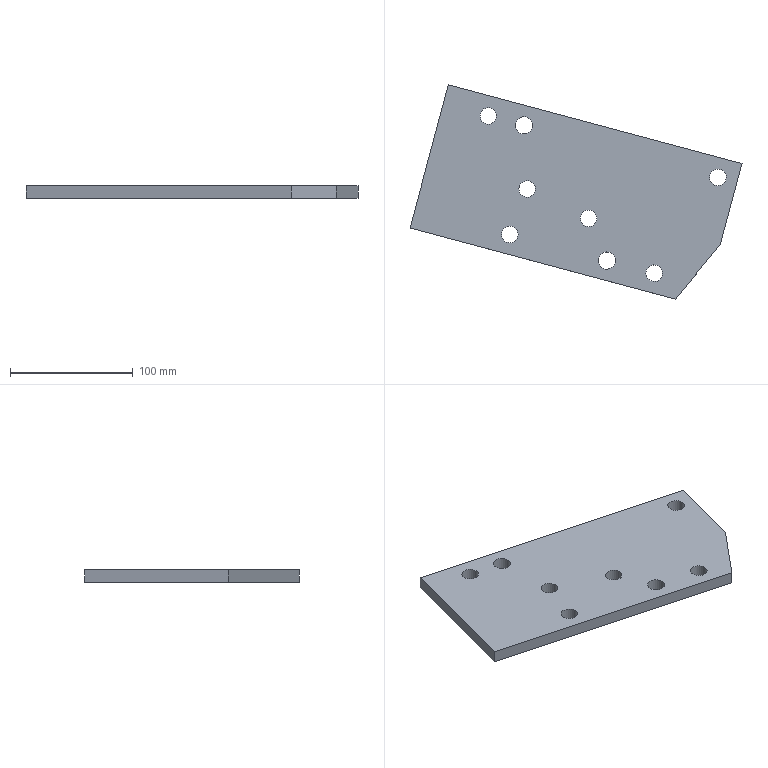Part | NX | features 6 2 | 1 solid | 15 faces | box 270.867 x 174.868 x 10 mm | volume 282148 mm3 | cylinder 8 | plane 7 | commonest cylinder face diameters 13.5 x6 14.001 x2
STEP:
#1=CARTESIAN_POINT('',(347.248,133.494,101.));
#2=VERTEX_POINT('',#1);
#3=CARTESIAN_POINT('',(315.931,16.617,101.));
#4=VERTEX_POINT('',#3);
#5=CARTESIAN_POINT('',(333.53,82.3,101.));
#6=DIRECTION('',(-0.2588,-0.9659,0.));
#7=VECTOR('',#6,1000.);
#8=LINE('',#5,#7);
#9=EDGE_CURVE('',#2,#4,#8,.T.);
#10=ORIENTED_EDGE('',*,*,#9,.T.);
#11=CARTESIAN_POINT('',(532.354,-41.373,101.));
#12=VERTEX_POINT('',#11);
#13=CARTESIAN_POINT('',(446.331,-18.323,101.));
#14=DIRECTION('',(0.9659,-0.2588,0.));
#15=VECTOR('',#14,1000.);
#16=LINE('',#13,#15);
#17=EDGE_CURVE('',#4,#12,#16,.T.);
#18=ORIENTED_EDGE('',*,*,#17,.T.);
#19=CARTESIAN_POINT('',(569.025,2.98,101.));
#20=VERTEX_POINT('',#19);
#21=CARTESIAN_POINT('',(291.39,-332.816,101.));
#22=DIRECTION('',(0.6372,0.7707,0.));
#23=VECTOR('',#22,1000.);
#24=LINE('',#21,#23);
#25=EDGE_CURVE('',#12,#20,#24,.T.);
#26=ORIENTED_EDGE('',*,*,#25,.T.);
#27=CARTESIAN_POINT('',(586.797,69.307,101.));
#28=VERTEX_POINT('',#27);
#29=CARTESIAN_POINT('',(573.08,18.113,101.));
#30=DIRECTION('',(0.2588,0.9659,0.));
#31=VECTOR('',#30,1000.);
#32=LINE('',#29,#31);
#33=EDGE_CURVE('',#20,#28,#32,.T.);
#34=ORIENTED_EDGE('',*,*,#33,.T.);
#35=CARTESIAN_POINT('',(477.648,98.554,101.));
#36=DIRECTION('',(-0.9659,0.2588,0.));
#37=VECTOR('',#36,1000.);
#38=LINE('',#35,#37);
#39=EDGE_CURVE('',#28,#2,#38,.T.);
#40=ORIENTED_EDGE('',*,*,#39,.T.);
#41=EDGE_LOOP('',(#10,#18,#26,#34,#40));
#42=FACE_BOUND('',#41,.T.);
#43=CARTESIAN_POINT('',(418.241,48.522,101.));
#44=VERTEX_POINT('',#43);
#45=CARTESIAN_POINT('',(411.491,48.522,101.));
#46=DIRECTION('',(0.,0.,1.));
#47=DIRECTION('',(1.,0.,0.));
#48=AXIS2_PLACEMENT_3D('',#45,#46,#47);
#49=CIRCLE('',#48,6.75);
#50=EDGE_CURVE('',#44,#44,#49,.T.);
#51=ORIENTED_EDGE('',*,*,#50,.F.);
#52=EDGE_LOOP('',(#51));
#53=FACE_BOUND('',#52,.T.);
#54=CARTESIAN_POINT('',(468.441,24.522,101.));
#55=VERTEX_POINT('',#54);
#56=CARTESIAN_POINT('',(461.691,24.522,101.));
#57=DIRECTION('',(0.,0.,1.));
#58=DIRECTION('',(1.,0.,0.));
#59=AXIS2_PLACEMENT_3D('',#56,#57,#58);
#60=CIRCLE('',#59,6.75);
#61=EDGE_CURVE('',#55,#55,#60,.T.);
#62=ORIENTED_EDGE('',*,*,#61,.F.);
#63=EDGE_LOOP('',(#62));
#64=FACE_BOUND('',#63,.T.);
#65=CARTESIAN_POINT('',(483.314,-11.668,101.));
#66=VERTEX_POINT('',#65);
#67=CARTESIAN_POINT('',(476.552,-9.857,101.));
#68=DIRECTION('',(0.,0.,1.));
#69=DIRECTION('',(0.9659,-0.2588,0.));
#70=AXIS2_PLACEMENT_3D('',#67,#68,#69);
#71=CIRCLE('',#70,7.);
#72=EDGE_CURVE('',#66,#66,#71,.T.);
#73=ORIENTED_EDGE('',*,*,#72,.F.);
#74=EDGE_LOOP('',(#73));
#75=FACE_BOUND('',#74,.T.);
#76=CARTESIAN_POINT('',(403.866,9.62,101.));
#77=VERTEX_POINT('',#76);
#78=CARTESIAN_POINT('',(397.346,11.367,101.));
#79=DIRECTION('',(0.,0.,1.));
#80=DIRECTION('',(0.9659,-0.2588,0.));
#81=AXIS2_PLACEMENT_3D('',#78,#79,#80);
#82=CIRCLE('',#81,6.75);
#83=EDGE_CURVE('',#77,#77,#82,.T.);
#84=ORIENTED_EDGE('',*,*,#83,.F.);
#85=EDGE_LOOP('',(#84));
#86=FACE_BOUND('',#85,.T.);
#87=CARTESIAN_POINT('',(521.709,-21.956,101.));
#88=VERTEX_POINT('',#87);
#89=CARTESIAN_POINT('',(515.189,-20.209,101.));
#90=DIRECTION('',(0.,0.,1.));
#91=DIRECTION('',(0.9659,-0.2588,0.));
#92=AXIS2_PLACEMENT_3D('',#89,#90,#91);
#93=CIRCLE('',#92,6.75);
#94=EDGE_CURVE('',#88,#88,#93,.T.);
#95=ORIENTED_EDGE('',*,*,#94,.F.);
#96=EDGE_LOOP('',(#95));
#97=FACE_BOUND('',#96,.T.);
#98=CARTESIAN_POINT('',(386.332,106.457,101.));
#99=VERTEX_POINT('',#98);
#100=CARTESIAN_POINT('',(379.812,108.204,101.));
#101=DIRECTION('',(0.,0.,1.));
#102=DIRECTION('',(0.9659,-0.2588,0.));
#103=AXIS2_PLACEMENT_3D('',#100,#101,#102);
#104=CIRCLE('',#103,6.75);
#105=EDGE_CURVE('',#99,#99,#104,.T.);
#106=ORIENTED_EDGE('',*,*,#105,.F.);
#107=EDGE_LOOP('',(#106));
#108=FACE_BOUND('',#107,.T.);
#109=CARTESIAN_POINT('',(573.721,56.246,101.));
#110=VERTEX_POINT('',#109);
#111=CARTESIAN_POINT('',(567.201,57.993,101.));
#112=DIRECTION('',(0.,0.,1.));
#113=DIRECTION('',(0.9659,-0.2588,0.));
#114=AXIS2_PLACEMENT_3D('',#111,#112,#113);
#115=CIRCLE('',#114,6.75);
#116=EDGE_CURVE('',#110,#110,#115,.T.);
#117=ORIENTED_EDGE('',*,*,#116,.F.);
#118=EDGE_LOOP('',(#117));
#119=FACE_BOUND('',#118,.T.);
#120=CARTESIAN_POINT('',(415.552,98.628,101.));
#121=VERTEX_POINT('',#120);
#122=CARTESIAN_POINT('',(408.79,100.44,101.));
#123=DIRECTION('',(0.,0.,1.));
#124=DIRECTION('',(0.9659,-0.2588,0.));
#125=AXIS2_PLACEMENT_3D('',#122,#123,#124);
#126=CIRCLE('',#125,7.);
#127=EDGE_CURVE('',#121,#121,#126,.T.);
#128=ORIENTED_EDGE('',*,*,#127,.F.);
#129=EDGE_LOOP('',(#128));
#130=FACE_BOUND('',#129,.T.);
#131=CARTESIAN_POINT('',(1.696,-93.298,101.));
#132=DIRECTION('',(0.,0.,1.));
#133=DIRECTION('',(-0.9848,-0.1736,0.));
#134=AXIS2_PLACEMENT_3D('',#131,#132,#133);
#135=PLANE('',#134);
#136=ADVANCED_FACE('',(#42,#53,#64,#75,#86,#97,#108,#119,#130),#135,.T.);
#137=CARTESIAN_POINT('',(532.354,-41.373,91.));
#138=VERTEX_POINT('',#137);
#139=CARTESIAN_POINT('',(315.931,16.617,91.));
#140=VERTEX_POINT('',#139);
#141=CARTESIAN_POINT('',(446.331,-18.323,91.));
#142=DIRECTION('',(-0.9659,0.2588,0.));
#143=VECTOR('',#142,1000.);
#144=LINE('',#141,#143);
#145=EDGE_CURVE('',#138,#140,#144,.T.);
#146=ORIENTED_EDGE('',*,*,#145,.T.);
#147=CARTESIAN_POINT('',(347.248,133.494,91.));
#148=VERTEX_POINT('',#147);
#149=CARTESIAN_POINT('',(333.53,82.3,91.));
#150=DIRECTION('',(0.2588,0.9659,0.));
#151=VECTOR('',#150,1000.);
#152=LINE('',#149,#151);
#153=EDGE_CURVE('',#140,#148,#152,.T.);
#154=ORIENTED_EDGE('',*,*,#153,.T.);
#155=CARTESIAN_POINT('',(586.797,69.307,91.));
#156=VERTEX_POINT('',#155);
#157=CARTESIAN_POINT('',(477.648,98.554,91.));
#158=DIRECTION('',(0.9659,-0.2588,0.));
#159=VECTOR('',#158,1000.);
#160=LINE('',#157,#159);
#161=EDGE_CURVE('',#148,#156,#160,.T.);
#162=ORIENTED_EDGE('',*,*,#161,.T.);
#163=CARTESIAN_POINT('',(569.025,2.98,91.));
#164=VERTEX_POINT('',#163);
#165=CARTESIAN_POINT('',(573.08,18.113,91.));
#166=DIRECTION('',(-0.2588,-0.9659,0.));
#167=VECTOR('',#166,1000.);
#168=LINE('',#165,#167);
#169=EDGE_CURVE('',#156,#164,#168,.T.);
#170=ORIENTED_EDGE('',*,*,#169,.T.);
#171=CARTESIAN_POINT('',(532.646,-41.021,91.));
#172=DIRECTION('',(0.6372,0.7707,0.));
#173=VECTOR('',#172,1000.);
#174=LINE('',#171,#173);
#175=EDGE_CURVE('',#138,#164,#174,.T.);
#176=ORIENTED_EDGE('',*,*,#175,.F.);
#177=EDGE_LOOP('',(#146,#154,#162,#170,#176));
#178=FACE_BOUND('',#177,.T.);
#179=CARTESIAN_POINT('',(415.552,98.628,91.));
#180=VERTEX_POINT('',#179);
#181=CARTESIAN_POINT('',(408.79,100.44,91.));
#182=DIRECTION('',(0.,0.,-1.));
#183=DIRECTION('',(0.9659,-0.2588,0.));
#184=AXIS2_PLACEMENT_3D('',#181,#182,#183);
#185=CIRCLE('',#184,7.);
#186=EDGE_CURVE('',#180,#180,#185,.T.);
#187=ORIENTED_EDGE('',*,*,#186,.F.);
#188=EDGE_LOOP('',(#187));
#189=FACE_BOUND('',#188,.T.);
#190=CARTESIAN_POINT('',(573.721,56.246,91.));
#191=VERTEX_POINT('',#190);
#192=CARTESIAN_POINT('',(567.201,57.993,91.));
#193=DIRECTION('',(0.,0.,-1.));
#194=DIRECTION('',(0.9659,-0.2588,0.));
#195=AXIS2_PLACEMENT_3D('',#192,#193,#194);
#196=CIRCLE('',#195,6.75);
#197=EDGE_CURVE('',#191,#191,#196,.T.);
#198=ORIENTED_EDGE('',*,*,#197,.F.);
#199=EDGE_LOOP('',(#198));
#200=FACE_BOUND('',#199,.T.);
#201=CARTESIAN_POINT('',(386.332,106.457,91.));
#202=VERTEX_POINT('',#201);
#203=CARTESIAN_POINT('',(379.812,108.204,91.));
#204=DIRECTION('',(0.,0.,-1.));
#205=DIRECTION('',(0.9659,-0.2588,0.));
#206=AXIS2_PLACEMENT_3D('',#203,#204,#205);
#207=CIRCLE('',#206,6.75);
#208=EDGE_CURVE('',#202,#202,#207,.T.);
#209=ORIENTED_EDGE('',*,*,#208,.F.);
#210=EDGE_LOOP('',(#209));
#211=FACE_BOUND('',#210,.T.);
#212=CARTESIAN_POINT('',(521.709,-21.956,91.));
#213=VERTEX_POINT('',#212);
#214=CARTESIAN_POINT('',(515.189,-20.209,91.));
#215=DIRECTION('',(0.,0.,-1.));
#216=DIRECTION('',(0.9659,-0.2588,0.));
#217=AXIS2_PLACEMENT_3D('',#214,#215,#216);
#218=CIRCLE('',#217,6.75);
#219=EDGE_CURVE('',#213,#213,#218,.T.);
#220=ORIENTED_EDGE('',*,*,#219,.F.);
#221=EDGE_LOOP('',(#220));
#222=FACE_BOUND('',#221,.T.);
#223=CARTESIAN_POINT('',(403.866,9.62,91.));
#224=VERTEX_POINT('',#223);
#225=CARTESIAN_POINT('',(397.346,11.367,91.));
#226=DIRECTION('',(0.,0.,-1.));
#227=DIRECTION('',(0.9659,-0.2588,0.));
#228=AXIS2_PLACEMENT_3D('',#225,#226,#227);
#229=CIRCLE('',#228,6.75);
#230=EDGE_CURVE('',#224,#224,#229,.T.);
#231=ORIENTED_EDGE('',*,*,#230,.F.);
#232=EDGE_LOOP('',(#231));
#233=FACE_BOUND('',#232,.T.);
#234=CARTESIAN_POINT('',(483.314,-11.668,91.));
#235=VERTEX_POINT('',#234);
#236=CARTESIAN_POINT('',(476.552,-9.857,91.));
#237=DIRECTION('',(0.,0.,-1.));
#238=DIRECTION('',(0.9659,-0.2588,0.));
#239=AXIS2_PLACEMENT_3D('',#236,#237,#238);
#240=CIRCLE('',#239,7.);
#241=EDGE_CURVE('',#235,#235,#240,.T.);
#242=ORIENTED_EDGE('',*,*,#241,.F.);
#243=EDGE_LOOP('',(#242));
#244=FACE_BOUND('',#243,.T.);
#245=CARTESIAN_POINT('',(454.941,24.522,91.));
#246=VERTEX_POINT('',#245);
#247=CARTESIAN_POINT('',(461.691,24.522,91.));
#248=DIRECTION('',(0.,0.,1.));
#249=DIRECTION('',(-1.,0.,0.));
#250=AXIS2_PLACEMENT_3D('',#247,#248,#249);
#251=CIRCLE('',#250,6.75);
#252=EDGE_CURVE('',#246,#246,#251,.T.);
#253=ORIENTED_EDGE('',*,*,#252,.T.);
#254=EDGE_LOOP('',(#253));
#255=FACE_BOUND('',#254,.T.);
#256=CARTESIAN_POINT('',(404.741,48.522,91.));
#257=VERTEX_POINT('',#256);
#258=CARTESIAN_POINT('',(411.491,48.522,91.));
#259=DIRECTION('',(0.,0.,1.));
#260=DIRECTION('',(-1.,0.,0.));
#261=AXIS2_PLACEMENT_3D('',#258,#259,#260);
#262=CIRCLE('',#261,6.75);
#263=EDGE_CURVE('',#257,#257,#262,.T.);
#264=ORIENTED_EDGE('',*,*,#263,.T.);
#265=EDGE_LOOP('',(#264));
#266=FACE_BOUND('',#265,.T.);
#267=CARTESIAN_POINT('',(463.93,47.36,91.));
#268=DIRECTION('',(0.,0.,-1.));
#269=DIRECTION('',(0.9659,-0.2588,0.));
#270=AXIS2_PLACEMENT_3D('',#267,#268,#269);
#271=PLANE('',#270);
#272=ADVANCED_FACE('',(#178,#189,#200,#211,#222,#233,#244,#255,#266),#271,.T.);
#273=ORIENTED_EDGE('',*,*,#17,.F.);
#274=CARTESIAN_POINT('',(315.931,16.617,91.));
#275=DIRECTION('',(0.,0.,1.));
#276=VECTOR('',#275,1000.);
#277=LINE('',#274,#276);
#278=EDGE_CURVE('',#140,#4,#277,.T.);
#279=ORIENTED_EDGE('',*,*,#278,.F.);
#280=ORIENTED_EDGE('',*,*,#145,.F.);
#281=CARTESIAN_POINT('',(532.354,-41.373,-36.));
#282=DIRECTION('',(0.,0.,-1.));
#283=VECTOR('',#282,1000.);
#284=LINE('',#281,#283);
#285=EDGE_CURVE('',#12,#138,#284,.T.);
#286=ORIENTED_EDGE('',*,*,#285,.F.);
#287=EDGE_LOOP('',(#273,#279,#280,#286));
#288=FACE_BOUND('',#287,.T.);
#289=CARTESIAN_POINT('',(446.331,-18.323,91.));
#290=DIRECTION('',(-0.2588,-0.9659,0.));
#291=DIRECTION('',(0.,0.,-1.));
#292=AXIS2_PLACEMENT_3D('',#289,#290,#291);
#293=PLANE('',#292);
#294=ADVANCED_FACE('',(#288),#293,.T.);
#295=ORIENTED_EDGE('',*,*,#153,.F.);
#296=ORIENTED_EDGE('',*,*,#278,.T.);
#297=ORIENTED_EDGE('',*,*,#9,.F.);
#298=CARTESIAN_POINT('',(347.248,133.494,91.));
#299=DIRECTION('',(0.,0.,1.));
#300=VECTOR('',#299,1000.);
#301=LINE('',#298,#300);
#302=EDGE_CURVE('',#148,#2,#301,.T.);
#303=ORIENTED_EDGE('',*,*,#302,.F.);
#304=EDGE_LOOP('',(#295,#296,#297,#303));
#305=FACE_BOUND('',#304,.T.);
#306=CARTESIAN_POINT('',(333.53,82.3,91.));
#307=DIRECTION('',(-0.9659,0.2588,0.));
#308=DIRECTION('',(0.,0.,-1.));
#309=AXIS2_PLACEMENT_3D('',#306,#307,#308);
#310=PLANE('',#309);
#311=ADVANCED_FACE('',(#305),#310,.T.);
#312=ORIENTED_EDGE('',*,*,#302,.T.);
#313=ORIENTED_EDGE('',*,*,#39,.F.);
#314=CARTESIAN_POINT('',(586.797,69.307,91.));
#315=DIRECTION('',(0.,0.,1.));
#316=VECTOR('',#315,1000.);
#317=LINE('',#314,#316);
#318=EDGE_CURVE('',#156,#28,#317,.T.);
#319=ORIENTED_EDGE('',*,*,#318,.F.);
#320=ORIENTED_EDGE('',*,*,#161,.F.);
#321=EDGE_LOOP('',(#312,#313,#319,#320));
#322=FACE_BOUND('',#321,.T.);
#323=CARTESIAN_POINT('',(477.648,98.554,91.));
#324=DIRECTION('',(0.2588,0.9659,0.));
#325=DIRECTION('',(0.,0.,1.));
#326=AXIS2_PLACEMENT_3D('',#323,#324,#325);
#327=PLANE('',#326);
#328=ADVANCED_FACE('',(#322),#327,.T.);
#329=ORIENTED_EDGE('',*,*,#33,.F.);
#330=CARTESIAN_POINT('',(569.025,2.98,-36.));
#331=DIRECTION('',(0.,0.,1.));
#332=VECTOR('',#331,1000.);
#333=LINE('',#330,#332);
#334=EDGE_CURVE('',#164,#20,#333,.T.);
#335=ORIENTED_EDGE('',*,*,#334,.F.);
#336=ORIENTED_EDGE('',*,*,#169,.F.);
#337=ORIENTED_EDGE('',*,*,#318,.T.);
#338=EDGE_LOOP('',(#329,#335,#336,#337));
#339=FACE_BOUND('',#338,.T.);
#340=CARTESIAN_POINT('',(573.08,18.113,91.));
#341=DIRECTION('',(0.9659,-0.2588,0.));
#342=DIRECTION('',(0.,0.,1.));
#343=AXIS2_PLACEMENT_3D('',#340,#341,#342);
#344=PLANE('',#343);
#345=ADVANCED_FACE('',(#339),#344,.T.);
#346=ORIENTED_EDGE('',*,*,#105,.T.);
#347=EDGE_LOOP('',(#346));
#348=FACE_BOUND('',#347,.T.);
#349=ORIENTED_EDGE('',*,*,#208,.T.);
#350=EDGE_LOOP('',(#349));
#351=FACE_BOUND('',#350,.T.);
#352=CARTESIAN_POINT('',(379.812,108.204,91.));
#353=DIRECTION('',(0.,0.,1.));
#354=DIRECTION('',(-0.9659,0.2588,0.));
#355=AXIS2_PLACEMENT_3D('',#352,#353,#354);
#356=CYLINDRICAL_SURFACE('',#355,6.75);
#357=ADVANCED_FACE('',(#348,#351),#356,.F.);
#358=ORIENTED_EDGE('',*,*,#94,.T.);
#359=EDGE_LOOP('',(#358));
#360=FACE_BOUND('',#359,.T.);
#361=ORIENTED_EDGE('',*,*,#219,.T.);
#362=EDGE_LOOP('',(#361));
#363=FACE_BOUND('',#362,.T.);
#364=CARTESIAN_POINT('',(515.189,-20.209,91.));
#365=DIRECTION('',(0.,0.,1.));
#366=DIRECTION('',(-0.9659,0.2588,0.));
#367=AXIS2_PLACEMENT_3D('',#364,#365,#366);
#368=CYLINDRICAL_SURFACE('',#367,6.75);
#369=ADVANCED_FACE('',(#360,#363),#368,.F.);
#370=ORIENTED_EDGE('',*,*,#116,.T.);
#371=EDGE_LOOP('',(#370));
#372=FACE_BOUND('',#371,.T.);
#373=ORIENTED_EDGE('',*,*,#197,.T.);
#374=EDGE_LOOP('',(#373));
#375=FACE_BOUND('',#374,.T.);
#376=CARTESIAN_POINT('',(567.201,57.993,91.));
#377=DIRECTION('',(0.,0.,1.));
#378=DIRECTION('',(-0.9659,0.2588,0.));
#379=AXIS2_PLACEMENT_3D('',#376,#377,#378);
#380=CYLINDRICAL_SURFACE('',#379,6.75);
#381=ADVANCED_FACE('',(#372,#375),#380,.F.);
#382=ORIENTED_EDGE('',*,*,#83,.T.);
#383=EDGE_LOOP('',(#382));
#384=FACE_BOUND('',#383,.T.);
#385=ORIENTED_EDGE('',*,*,#230,.T.);
#386=EDGE_LOOP('',(#385));
#387=FACE_BOUND('',#386,.T.);
#388=CARTESIAN_POINT('',(397.346,11.367,91.));
#389=DIRECTION('',(0.,0.,1.));
#390=DIRECTION('',(-0.9659,0.2588,0.));
#391=AXIS2_PLACEMENT_3D('',#388,#389,#390);
#392=CYLINDRICAL_SURFACE('',#391,6.75);
#393=ADVANCED_FACE('',(#384,#387),#392,.F.);
#394=ORIENTED_EDGE('',*,*,#127,.T.);
#395=EDGE_LOOP('',(#394));
#396=FACE_BOUND('',#395,.T.);
#397=ORIENTED_EDGE('',*,*,#186,.T.);
#398=EDGE_LOOP('',(#397));
#399=FACE_BOUND('',#398,.T.);
#400=CARTESIAN_POINT('',(408.79,100.44,91.));
#401=DIRECTION('',(0.,0.,1.));
#402=DIRECTION('',(-0.9659,0.2588,0.));
#403=AXIS2_PLACEMENT_3D('',#400,#401,#402);
#404=CYLINDRICAL_SURFACE('',#403,7.);
#405=ADVANCED_FACE('',(#396,#399),#404,.F.);
#406=ORIENTED_EDGE('',*,*,#72,.T.);
#407=EDGE_LOOP('',(#406));
#408=FACE_BOUND('',#407,.T.);
#409=ORIENTED_EDGE('',*,*,#241,.T.);
#410=EDGE_LOOP('',(#409));
#411=FACE_BOUND('',#410,.T.);
#412=CARTESIAN_POINT('',(476.552,-9.857,91.));
#413=DIRECTION('',(0.,0.,1.));
#414=DIRECTION('',(-0.9659,0.2588,0.));
#415=AXIS2_PLACEMENT_3D('',#412,#413,#414);
#416=CYLINDRICAL_SURFACE('',#415,7.);
#417=ADVANCED_FACE('',(#408,#411),#416,.F.);
#418=ORIENTED_EDGE('',*,*,#25,.F.);
#419=ORIENTED_EDGE('',*,*,#285,.T.);
#420=ORIENTED_EDGE('',*,*,#175,.T.);
#421=ORIENTED_EDGE('',*,*,#334,.T.);
#422=EDGE_LOOP('',(#418,#419,#420,#421));
#423=FACE_BOUND('',#422,.T.);
#424=CARTESIAN_POINT('',(532.646,-41.021,-36.));
#425=DIRECTION('',(0.7707,-0.6372,0.));
#426=DIRECTION('',(-0.6372,-0.7707,0.));
#427=AXIS2_PLACEMENT_3D('',#424,#425,#426);
#428=PLANE('',#427);
#429=ADVANCED_FACE('',(#423),#428,.T.);
#430=ORIENTED_EDGE('',*,*,#61,.T.);
#431=EDGE_LOOP('',(#430));
#432=FACE_BOUND('',#431,.T.);
#433=ORIENTED_EDGE('',*,*,#252,.F.);
#434=EDGE_LOOP('',(#433));
#435=FACE_BOUND('',#434,.T.);
#436=CARTESIAN_POINT('',(461.691,24.522,-61.));
#437=DIRECTION('',(0.,0.,1.));
#438=DIRECTION('',(-1.,0.,0.));
#439=AXIS2_PLACEMENT_3D('',#436,#437,#438);
#440=CYLINDRICAL_SURFACE('',#439,6.75);
#441=ADVANCED_FACE('',(#432,#435),#440,.F.);
#442=ORIENTED_EDGE('',*,*,#50,.T.);
#443=EDGE_LOOP('',(#442));
#444=FACE_BOUND('',#443,.T.);
#445=ORIENTED_EDGE('',*,*,#263,.F.);
#446=EDGE_LOOP('',(#445));
#447=FACE_BOUND('',#446,.T.);
#448=CARTESIAN_POINT('',(411.491,48.522,-61.));
#449=DIRECTION('',(0.,0.,1.));
#450=DIRECTION('',(-1.,0.,0.));
#451=AXIS2_PLACEMENT_3D('',#448,#449,#450);
#452=CYLINDRICAL_SURFACE('',#451,6.75);
#453=ADVANCED_FACE('',(#444,#447),#452,.F.);
#454=CLOSED_SHELL('',(#136,#272,#294,#311,#328,#345,#357,#369,#381,#393,#405,#417,#429,#441,#453));
#455=MANIFOLD_SOLID_BREP('',#454);
#456=(LENGTH_UNIT()NAMED_UNIT(*)SI_UNIT(.MILLI.,.METRE.));
#457=UNCERTAINTY_MEASURE_WITH_UNIT(LENGTH_MEASURE(0.00001),#456,'','');
#458=(NAMED_UNIT(*)PLANE_ANGLE_UNIT()SI_UNIT($,.RADIAN.));
#459=(NAMED_UNIT(*)SI_UNIT($,.STERADIAN.)SOLID_ANGLE_UNIT());
#460=(GEOMETRIC_REPRESENTATION_CONTEXT(3)GLOBAL_UNCERTAINTY_ASSIGNED_CONTEXT((#457))GLOBAL_UNIT_ASSIGNED_CONTEXT((#456,#458,#459))REPRESENTATION_CONTEXT('',''));
#461=ADVANCED_BREP_SHAPE_REPRESENTATION('',(#455),#460);